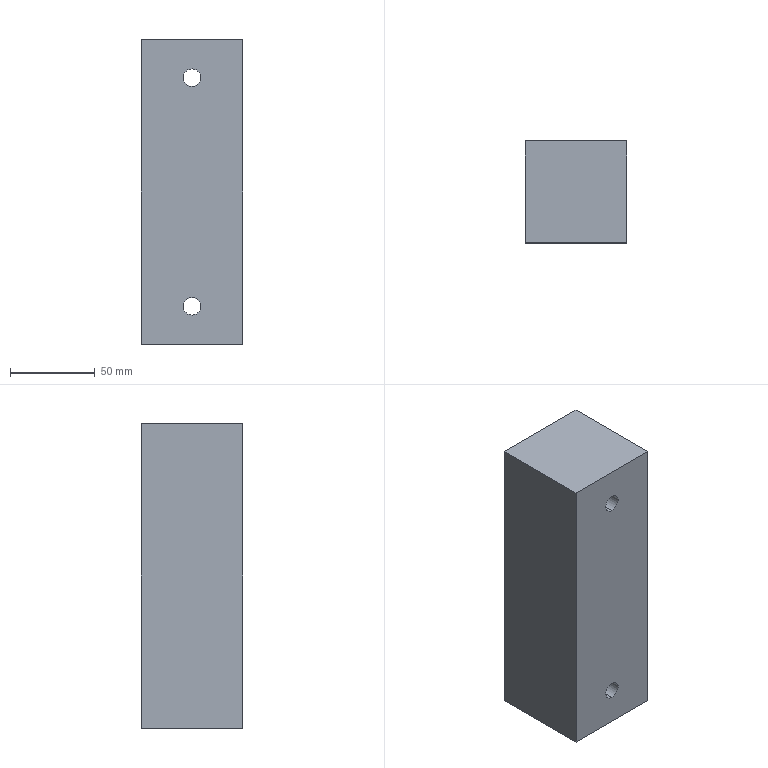Part | SolidWorks | features Extrusion 1, HoleWzd 1 | 1 solid | 10 faces | box 60 x 60 x 180 mm | volume 638194 mm3 | plane 6 | cylinder 4 | commonest cylinder face diameters 10.2 x4
STEP:
#1=CARTESIAN_POINT('',(0.,-30.,17.4));
#2=VERTEX_POINT('',#1);
#3=CARTESIAN_POINT('',(0.,-30.,27.6));
#4=VERTEX_POINT('',#3);
#5=CARTESIAN_POINT('',(0.,-30.,22.5));
#6=DIRECTION('',(0.,1.,0.));
#7=DIRECTION('',(0.,0.,1.));
#8=AXIS2_PLACEMENT_3D('',#5,#6,#7);
#9=CIRCLE('',#8,5.1);
#10=EDGE_CURVE('',#2,#4,#9,.T.);
#11=ORIENTED_EDGE('',*,*,#10,.F.);
#12=CARTESIAN_POINT('',(0.,30.,17.4));
#13=VERTEX_POINT('',#12);
#14=CARTESIAN_POINT('',(0.,30.,17.4));
#15=DIRECTION('',(0.,1.,0.));
#16=VECTOR('',#15,1000.);
#17=LINE('',#14,#16);
#18=EDGE_CURVE('',#2,#13,#17,.T.);
#19=ORIENTED_EDGE('',*,*,#18,.T.);
#20=CARTESIAN_POINT('',(0.,30.,27.6));
#21=VERTEX_POINT('',#20);
#22=CARTESIAN_POINT('',(0.,30.,22.5));
#23=DIRECTION('',(0.,1.,0.));
#24=DIRECTION('',(0.,0.,1.));
#25=AXIS2_PLACEMENT_3D('',#22,#23,#24);
#26=CIRCLE('',#25,5.1);
#27=EDGE_CURVE('',#13,#21,#26,.T.);
#28=ORIENTED_EDGE('',*,*,#27,.T.);
#29=CARTESIAN_POINT('',(0.,30.,27.6));
#30=DIRECTION('',(0.,1.,0.));
#31=VECTOR('',#30,1000.);
#32=LINE('',#29,#31);
#33=EDGE_CURVE('',#4,#21,#32,.T.);
#34=ORIENTED_EDGE('',*,*,#33,.F.);
#35=EDGE_LOOP('',(#11,#19,#28,#34));
#36=FACE_OUTER_BOUND('',#35,.T.);
#37=CARTESIAN_POINT('',(0.,30.,22.5));
#38=DIRECTION('',(0.,1.,0.));
#39=DIRECTION('',(0.,0.,1.));
#40=AXIS2_PLACEMENT_3D('',#37,#38,#39);
#41=CYLINDRICAL_SURFACE('',#40,5.1);
#42=ADVANCED_FACE('',(#36),#41,.F.);
#43=CARTESIAN_POINT('',(0.,-30.,152.4));
#44=VERTEX_POINT('',#43);
#45=CARTESIAN_POINT('',(0.,-30.,162.6));
#46=VERTEX_POINT('',#45);
#47=CARTESIAN_POINT('',(0.,-30.,157.5));
#48=DIRECTION('',(0.,1.,0.));
#49=DIRECTION('',(0.,0.,1.));
#50=AXIS2_PLACEMENT_3D('',#47,#48,#49);
#51=CIRCLE('',#50,5.1);
#52=EDGE_CURVE('',#44,#46,#51,.T.);
#53=ORIENTED_EDGE('',*,*,#52,.F.);
#54=CARTESIAN_POINT('',(0.,30.,152.4));
#55=VERTEX_POINT('',#54);
#56=CARTESIAN_POINT('',(0.,30.,152.4));
#57=DIRECTION('',(0.,1.,0.));
#58=VECTOR('',#57,1000.);
#59=LINE('',#56,#58);
#60=EDGE_CURVE('',#44,#55,#59,.T.);
#61=ORIENTED_EDGE('',*,*,#60,.T.);
#62=CARTESIAN_POINT('',(0.,30.,162.6));
#63=VERTEX_POINT('',#62);
#64=CARTESIAN_POINT('',(0.,30.,157.5));
#65=DIRECTION('',(0.,1.,0.));
#66=DIRECTION('',(0.,0.,1.));
#67=AXIS2_PLACEMENT_3D('',#64,#65,#66);
#68=CIRCLE('',#67,5.1);
#69=EDGE_CURVE('',#55,#63,#68,.T.);
#70=ORIENTED_EDGE('',*,*,#69,.T.);
#71=CARTESIAN_POINT('',(0.,30.,162.6));
#72=DIRECTION('',(0.,1.,0.));
#73=VECTOR('',#72,1000.);
#74=LINE('',#71,#73);
#75=EDGE_CURVE('',#46,#63,#74,.T.);
#76=ORIENTED_EDGE('',*,*,#75,.F.);
#77=EDGE_LOOP('',(#53,#61,#70,#76));
#78=FACE_OUTER_BOUND('',#77,.T.);
#79=CARTESIAN_POINT('',(0.,30.,157.5));
#80=DIRECTION('',(0.,1.,0.));
#81=DIRECTION('',(0.,0.,1.));
#82=AXIS2_PLACEMENT_3D('',#79,#80,#81);
#83=CYLINDRICAL_SURFACE('',#82,5.1);
#84=ADVANCED_FACE('',(#78),#83,.F.);
#85=CARTESIAN_POINT('',(-30.,30.,0.));
#86=VERTEX_POINT('',#85);
#87=CARTESIAN_POINT('',(-30.,-30.,0.));
#88=VERTEX_POINT('',#87);
#89=CARTESIAN_POINT('',(-30.,30.,0.));
#90=DIRECTION('',(0.,-1.,0.));
#91=VECTOR('',#90,1000.);
#92=LINE('',#89,#91);
#93=EDGE_CURVE('',#86,#88,#92,.T.);
#94=ORIENTED_EDGE('',*,*,#93,.T.);
#95=CARTESIAN_POINT('',(-30.,-30.,180.));
#96=VERTEX_POINT('',#95);
#97=CARTESIAN_POINT('',(-30.,-30.,180.));
#98=DIRECTION('',(0.,0.,-1.));
#99=VECTOR('',#98,1000.);
#100=LINE('',#97,#99);
#101=EDGE_CURVE('',#96,#88,#100,.T.);
#102=ORIENTED_EDGE('',*,*,#101,.F.);
#103=CARTESIAN_POINT('',(-30.,30.,180.));
#104=VERTEX_POINT('',#103);
#105=CARTESIAN_POINT('',(-30.,30.,180.));
#106=DIRECTION('',(0.,-1.,0.));
#107=VECTOR('',#106,1000.);
#108=LINE('',#105,#107);
#109=EDGE_CURVE('',#104,#96,#108,.T.);
#110=ORIENTED_EDGE('',*,*,#109,.F.);
#111=CARTESIAN_POINT('',(-30.,30.,180.));
#112=DIRECTION('',(0.,0.,-1.));
#113=VECTOR('',#112,1000.);
#114=LINE('',#111,#113);
#115=EDGE_CURVE('',#104,#86,#114,.T.);
#116=ORIENTED_EDGE('',*,*,#115,.T.);
#117=EDGE_LOOP('',(#94,#102,#110,#116));
#118=FACE_OUTER_BOUND('',#117,.T.);
#119=CARTESIAN_POINT('',(-30.,30.,180.));
#120=DIRECTION('',(1.,0.,0.));
#121=DIRECTION('',(0.,1.,0.));
#122=AXIS2_PLACEMENT_3D('',#119,#120,#121);
#123=PLANE('',#122);
#124=ADVANCED_FACE('',(#118),#123,.F.);
#125=CARTESIAN_POINT('',(0.,-30.,22.5));
#126=DIRECTION('',(0.,1.,0.));
#127=DIRECTION('',(0.,0.,1.));
#128=AXIS2_PLACEMENT_3D('',#125,#126,#127);
#129=CIRCLE('',#128,5.1);
#130=EDGE_CURVE('',#4,#2,#129,.T.);
#131=ORIENTED_EDGE('',*,*,#130,.T.);
#132=ORIENTED_EDGE('',*,*,#10,.T.);
#133=EDGE_LOOP('',(#131,#132));
#134=FACE_BOUND('',#133,.T.);
#135=CARTESIAN_POINT('',(0.,-30.,157.5));
#136=DIRECTION('',(0.,1.,0.));
#137=DIRECTION('',(0.,0.,1.));
#138=AXIS2_PLACEMENT_3D('',#135,#136,#137);
#139=CIRCLE('',#138,5.1);
#140=EDGE_CURVE('',#46,#44,#139,.T.);
#141=ORIENTED_EDGE('',*,*,#140,.T.);
#142=ORIENTED_EDGE('',*,*,#52,.T.);
#143=EDGE_LOOP('',(#141,#142));
#144=FACE_BOUND('',#143,.T.);
#145=CARTESIAN_POINT('',(30.,-30.,0.));
#146=VERTEX_POINT('',#145);
#147=CARTESIAN_POINT('',(30.,-30.,0.));
#148=DIRECTION('',(1.,0.,0.));
#149=VECTOR('',#148,1000.);
#150=LINE('',#147,#149);
#151=EDGE_CURVE('',#88,#146,#150,.T.);
#152=ORIENTED_EDGE('',*,*,#151,.T.);
#153=CARTESIAN_POINT('',(30.,-30.,180.));
#154=VERTEX_POINT('',#153);
#155=CARTESIAN_POINT('',(30.,-30.,180.));
#156=DIRECTION('',(0.,0.,-1.));
#157=VECTOR('',#156,1000.);
#158=LINE('',#155,#157);
#159=EDGE_CURVE('',#154,#146,#158,.T.);
#160=ORIENTED_EDGE('',*,*,#159,.F.);
#161=CARTESIAN_POINT('',(30.,-30.,180.));
#162=DIRECTION('',(1.,0.,0.));
#163=VECTOR('',#162,1000.);
#164=LINE('',#161,#163);
#165=EDGE_CURVE('',#96,#154,#164,.T.);
#166=ORIENTED_EDGE('',*,*,#165,.F.);
#167=ORIENTED_EDGE('',*,*,#101,.T.);
#168=EDGE_LOOP('',(#152,#160,#166,#167));
#169=FACE_OUTER_BOUND('',#168,.T.);
#170=CARTESIAN_POINT('',(30.,-30.,180.));
#171=DIRECTION('',(0.,1.,0.));
#172=DIRECTION('',(-1.,0.,0.));
#173=AXIS2_PLACEMENT_3D('',#170,#171,#172);
#174=PLANE('',#173);
#175=ADVANCED_FACE('',(#134,#144,#169),#174,.F.);
#176=CARTESIAN_POINT('',(30.,30.,0.));
#177=VERTEX_POINT('',#176);
#178=CARTESIAN_POINT('',(30.,30.,0.));
#179=DIRECTION('',(0.,1.,0.));
#180=VECTOR('',#179,1000.);
#181=LINE('',#178,#180);
#182=EDGE_CURVE('',#146,#177,#181,.T.);
#183=ORIENTED_EDGE('',*,*,#182,.T.);
#184=CARTESIAN_POINT('',(30.,30.,180.));
#185=VERTEX_POINT('',#184);
#186=CARTESIAN_POINT('',(30.,30.,180.));
#187=DIRECTION('',(0.,0.,-1.));
#188=VECTOR('',#187,1000.);
#189=LINE('',#186,#188);
#190=EDGE_CURVE('',#185,#177,#189,.T.);
#191=ORIENTED_EDGE('',*,*,#190,.F.);
#192=CARTESIAN_POINT('',(30.,30.,180.));
#193=DIRECTION('',(0.,1.,0.));
#194=VECTOR('',#193,1000.);
#195=LINE('',#192,#194);
#196=EDGE_CURVE('',#154,#185,#195,.T.);
#197=ORIENTED_EDGE('',*,*,#196,.F.);
#198=ORIENTED_EDGE('',*,*,#159,.T.);
#199=EDGE_LOOP('',(#183,#191,#197,#198));
#200=FACE_OUTER_BOUND('',#199,.T.);
#201=CARTESIAN_POINT('',(30.,30.,180.));
#202=DIRECTION('',(-1.,0.,0.));
#203=DIRECTION('',(0.,-1.,0.));
#204=AXIS2_PLACEMENT_3D('',#201,#202,#203);
#205=PLANE('',#204);
#206=ADVANCED_FACE('',(#200),#205,.F.);
#207=CARTESIAN_POINT('',(0.,30.,22.5));
#208=DIRECTION('',(0.,1.,0.));
#209=DIRECTION('',(0.,0.,1.));
#210=AXIS2_PLACEMENT_3D('',#207,#208,#209);
#211=CIRCLE('',#210,5.1);
#212=EDGE_CURVE('',#21,#13,#211,.T.);
#213=ORIENTED_EDGE('',*,*,#212,.F.);
#214=ORIENTED_EDGE('',*,*,#27,.F.);
#215=EDGE_LOOP('',(#213,#214));
#216=FACE_BOUND('',#215,.T.);
#217=CARTESIAN_POINT('',(0.,30.,157.5));
#218=DIRECTION('',(0.,1.,0.));
#219=DIRECTION('',(0.,0.,1.));
#220=AXIS2_PLACEMENT_3D('',#217,#218,#219);
#221=CIRCLE('',#220,5.1);
#222=EDGE_CURVE('',#63,#55,#221,.T.);
#223=ORIENTED_EDGE('',*,*,#222,.F.);
#224=ORIENTED_EDGE('',*,*,#69,.F.);
#225=EDGE_LOOP('',(#223,#224));
#226=FACE_BOUND('',#225,.T.);
#227=CARTESIAN_POINT('',(30.,30.,0.));
#228=DIRECTION('',(-1.,0.,0.));
#229=VECTOR('',#228,1000.);
#230=LINE('',#227,#229);
#231=EDGE_CURVE('',#177,#86,#230,.T.);
#232=ORIENTED_EDGE('',*,*,#231,.T.);
#233=ORIENTED_EDGE('',*,*,#115,.F.);
#234=CARTESIAN_POINT('',(30.,30.,180.));
#235=DIRECTION('',(-1.,0.,0.));
#236=VECTOR('',#235,1000.);
#237=LINE('',#234,#236);
#238=EDGE_CURVE('',#185,#104,#237,.T.);
#239=ORIENTED_EDGE('',*,*,#238,.F.);
#240=ORIENTED_EDGE('',*,*,#190,.T.);
#241=EDGE_LOOP('',(#232,#233,#239,#240));
#242=FACE_OUTER_BOUND('',#241,.T.);
#243=CARTESIAN_POINT('',(30.,30.,180.));
#244=DIRECTION('',(0.,-1.,0.));
#245=DIRECTION('',(1.,0.,0.));
#246=AXIS2_PLACEMENT_3D('',#243,#244,#245);
#247=PLANE('',#246);
#248=ADVANCED_FACE('',(#216,#226,#242),#247,.F.);
#249=ORIENTED_EDGE('',*,*,#109,.T.);
#250=ORIENTED_EDGE('',*,*,#165,.T.);
#251=ORIENTED_EDGE('',*,*,#196,.T.);
#252=ORIENTED_EDGE('',*,*,#238,.T.);
#253=EDGE_LOOP('',(#249,#250,#251,#252));
#254=FACE_OUTER_BOUND('',#253,.T.);
#255=CARTESIAN_POINT('',(0.,0.,180.));
#256=DIRECTION('',(0.,0.,-1.));
#257=DIRECTION('',(-1.,0.,0.));
#258=AXIS2_PLACEMENT_3D('',#255,#256,#257);
#259=PLANE('',#258);
#260=ADVANCED_FACE('',(#254),#259,.F.);
#261=ORIENTED_EDGE('',*,*,#93,.F.);
#262=ORIENTED_EDGE('',*,*,#231,.F.);
#263=ORIENTED_EDGE('',*,*,#182,.F.);
#264=ORIENTED_EDGE('',*,*,#151,.F.);
#265=EDGE_LOOP('',(#261,#262,#263,#264));
#266=FACE_OUTER_BOUND('',#265,.T.);
#267=CARTESIAN_POINT('',(0.,0.,0.));
#268=DIRECTION('',(0.,0.,-1.));
#269=DIRECTION('',(-1.,0.,0.));
#270=AXIS2_PLACEMENT_3D('',#267,#268,#269);
#271=PLANE('',#270);
#272=ADVANCED_FACE('',(#266),#271,.T.);
#273=ORIENTED_EDGE('',*,*,#60,.F.);
#274=ORIENTED_EDGE('',*,*,#140,.F.);
#275=ORIENTED_EDGE('',*,*,#75,.T.);
#276=ORIENTED_EDGE('',*,*,#222,.T.);
#277=EDGE_LOOP('',(#273,#274,#275,#276));
#278=FACE_OUTER_BOUND('',#277,.T.);
#279=CARTESIAN_POINT('',(0.,30.,157.5));
#280=DIRECTION('',(0.,1.,0.));
#281=DIRECTION('',(0.,0.,1.));
#282=AXIS2_PLACEMENT_3D('',#279,#280,#281);
#283=CYLINDRICAL_SURFACE('',#282,5.1);
#284=ADVANCED_FACE('',(#278),#283,.F.);
#285=ORIENTED_EDGE('',*,*,#18,.F.);
#286=ORIENTED_EDGE('',*,*,#130,.F.);
#287=ORIENTED_EDGE('',*,*,#33,.T.);
#288=ORIENTED_EDGE('',*,*,#212,.T.);
#289=EDGE_LOOP('',(#285,#286,#287,#288));
#290=FACE_OUTER_BOUND('',#289,.T.);
#291=CARTESIAN_POINT('',(0.,30.,22.5));
#292=DIRECTION('',(0.,1.,0.));
#293=DIRECTION('',(0.,0.,1.));
#294=AXIS2_PLACEMENT_3D('',#291,#292,#293);
#295=CYLINDRICAL_SURFACE('',#294,5.1);
#296=ADVANCED_FACE('',(#290),#295,.F.);
#297=CLOSED_SHELL('',(#42,#84,#124,#175,#206,#248,#260,#272,#284,#296));
#298=MANIFOLD_SOLID_BREP('',#297);
#299=CARTESIAN_POINT('',(0.,0.,0.));
#300=DIRECTION('',(0.,0.,1.));
#301=DIRECTION('',(1.,0.,0.));
#302=AXIS2_PLACEMENT_3D('',#299,#300,#301);
#303=(LENGTH_UNIT()NAMED_UNIT(*)SI_UNIT(.MILLI.,.METRE.));
#304=UNCERTAINTY_MEASURE_WITH_UNIT(LENGTH_MEASURE(0.00001),#303,'','');
#305=(NAMED_UNIT(*)PLANE_ANGLE_UNIT()SI_UNIT($,.RADIAN.));
#306=(NAMED_UNIT(*)SI_UNIT($,.STERADIAN.)SOLID_ANGLE_UNIT());
#307=(GEOMETRIC_REPRESENTATION_CONTEXT(3)GLOBAL_UNCERTAINTY_ASSIGNED_CONTEXT((#304))GLOBAL_UNIT_ASSIGNED_CONTEXT((#303,#305,#306))REPRESENTATION_CONTEXT('',''));
#308=ADVANCED_BREP_SHAPE_REPRESENTATION('',(#298,#302),#307);